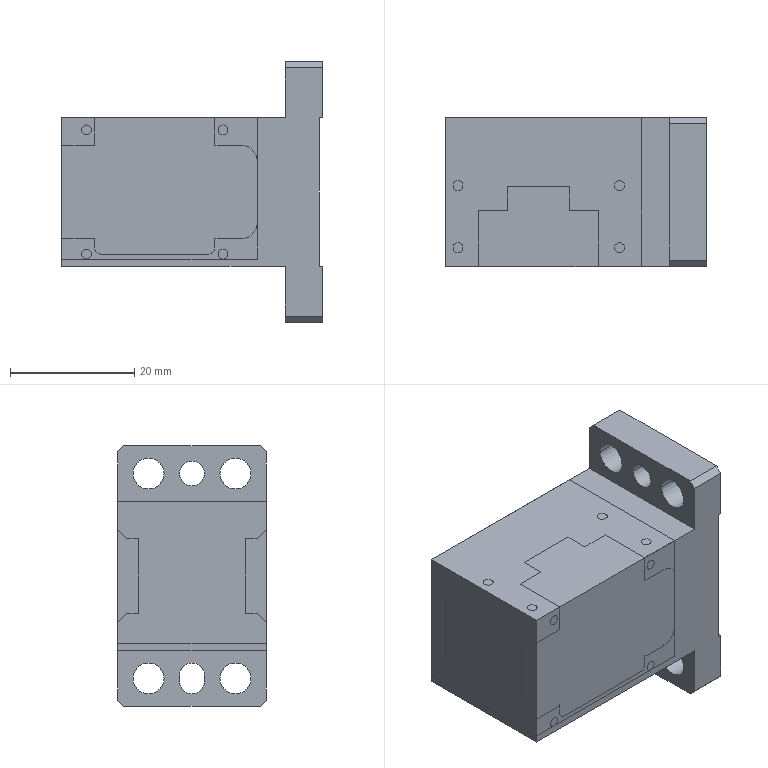NC program | NX | posted with a generic post | part box 42 x 24 x 42 mm
Lines 19 to 1216 of 4089:
(ZLEVEL_PROFILE , TOOL : D10)
N36 T10 M6
N38 G54
N40 G17 G0 G90 X26.1 Y11.429 B0. C0. S3000 M3
N42 G43 Z30. H10
N44 Z1.5
N46 G94 G1 Y-12. Z0.272 F1000.
N48 Y-12.554 Z0.243
N50 X25.766 Y-13.898 Z0.171
N52 X25.084 Y-15.104 Z0.098
N54 X24.104 Y-16.084 Z0.025
N56 X22.898 Y-16.766 Z-0.047
N58 X21.554 Y-17.1 Z-0.12
N60 X21. Z-0.149
N62 X-21. F1800.
N64 G2 X-26.1 Y-12. R5.1
N66 G1 Y12.
N68 G2 X-21. Y17.1 R5.1
N70 G1 X21.
N72 G2 X26.1 Y12. R5.1
N74 G1 Y-12.
N76 G2 X21. Y-17.1 R5.1
N78 G1 X12.467 Z-0.298
N80 X-21.
N82 G2 X-26.1 Y-12. R5.1
N84 G1 Y12.
N86 G2 X-21. Y17.1 R5.1
N88 G1 X21.
N90 G2 X26.1 Y12. R5.1
N92 G1 Y-12.
N94 G2 X21. Y-17.1 R5.1
N96 G1 X12.467 Z-0.447
N98 X-21.
N100 G2 X-26.1 Y-12. R5.1
N102 G1 Y12.
N104 G2 X-21. Y17.1 R5.1
N106 G1 X21.
N108 G2 X26.1 Y12. R5.1
N110 G1 Y-12.
N112 G2 X21. Y-17.1 R5.1
N114 G1 X12.467 Z-0.596
N116 X-21.
N118 G2 X-26.1 Y-12. R5.1
N120 G1 Y12.
N122 G2 X-21. Y17.1 R5.1
N124 G1 X21.
N126 G2 X26.1 Y12. R5.1
N128 G1 Y-12.
N130 G2 X21. Y-17.1 R5.1
N132 G1 X12.467 Z-0.745
N134 X-21.
N136 G2 X-26.1 Y-12. R5.1
N138 G1 Y12.
N140 G2 X-21. Y17.1 R5.1
N142 G1 X21.
N144 G2 X26.1 Y12. R5.1
N146 G1 Y-12.
N148 G2 X21. Y-17.1 R5.1
N150 G1 X12.467 Z-0.894
N152 X-21.
N154 G2 X-26.1 Y-12. R5.1
N156 G1 Y12.
N158 G2 X-21. Y17.1 R5.1
N160 G1 X21.
N162 G2 X26.1 Y12. R5.1
N164 G1 Y-12.
N166 G2 X21. Y-17.1 R5.1
N168 G1 X12.467 Z-1.043
N170 X-21.
N172 G2 X-26.1 Y-12. R5.1
N174 G1 Y12.
N176 G2 X-21. Y17.1 R5.1
N178 G1 X21.
N180 G2 X26.1 Y12. R5.1
N182 G1 Y-12.
N184 G2 X21. Y-17.1 R5.1
N186 G1 X12.467 Z-1.191
N188 X-21.
N190 G2 X-26.1 Y-12. R5.1
N192 G1 Y12.
N194 G2 X-21. Y17.1 R5.1
N196 G1 X21.
N198 G2 X26.1 Y12. R5.1
N200 G1 Y-12.
N202 G2 X21. Y-17.1 R5.1
N204 G1 X12.467 Z-1.34
N206 X-21.
N208 G2 X-26.1 Y-12. R5.1
N210 G1 Y12.
N212 G2 X-21. Y17.1 R5.1
N214 G1 X21.
N216 G2 X26.1 Y12. R5.1
N218 G1 Y-12.
N220 G2 X21. Y-17.1 R5.1
N222 G1 X12.467 Z-1.489
N224 X-21.
N226 G2 X-26.1 Y-12. R5.1
N228 G1 Y12.
N230 G2 X-21. Y17.1 R5.1
N232 G1 X21.
N234 G2 X26.1 Y12. R5.1
N236 G1 Y-12.
N238 G2 X21. Y-17.1 R5.1
N240 G1 X12.467 Z-1.638
N242 X-21.
N244 G2 X-26.1 Y-12. R5.1
N246 G1 Y12.
N248 G2 X-21. Y17.1 R5.1
N250 G1 X21.
N252 G2 X26.1 Y12. R5.1
N254 G1 Y-12.
N256 G2 X21. Y-17.1 R5.1
N258 G1 X12.467 Z-1.787
N260 X-21.
N262 G2 X-26.1 Y-12. R5.1
N264 G1 Y12.
N266 G2 X-21. Y17.1 R5.1
N268 G1 X21.
N270 G2 X26.1 Y12. R5.1
N272 G1 Y-12.
N274 G2 X21. Y-17.1 R5.1
N276 G1 X12.467 Z-1.936
N278 X-21.
N280 G2 X-26.1 Y-12. R5.1
N282 G1 Y12.
N284 G2 X-21. Y17.1 R5.1
N286 G1 X21.
N288 G2 X26.1 Y12. R5.1
N290 G1 Y-12.
N292 G2 X21. Y-17.1 R5.1
N294 G1 X12.467 Z-2.085
N296 X-21.
N298 G2 X-26.1 Y-12. R5.1
N300 G1 Y12.
N302 G2 X-21. Y17.1 R5.1
N304 G1 X21.
N306 G2 X26.1 Y12. R5.1
N308 G1 Y-12.
N310 G2 X21. Y-17.1 R5.1
N312 G1 X12.467 Z-2.234
N314 X-21.
N316 G2 X-26.1 Y-12. R5.1
N318 G1 Y12.
N320 G2 X-21. Y17.1 R5.1
N322 G1 X21.
N324 G2 X26.1 Y12. R5.1
N326 G1 Y-12.
N328 G2 X21. Y-17.1 R5.1
N330 G1 X12.467 Z-2.383
N332 X-21.
N334 G2 X-26.1 Y-12. R5.1
N336 G1 Y12.
N338 G2 X-21. Y17.1 R5.1
N340 G1 X21.
N342 G2 X26.1 Y12. R5.1
N344 G1 Y-12.
N346 G2 X21. Y-17.1 R5.1
N348 G1 X12.467 Z-2.532
N350 X-21.
N352 G2 X-26.1 Y-12. R5.1
N354 G1 Y12.
N356 G2 X-21. Y17.1 R5.1
N358 G1 X21.
N360 G2 X26.1 Y12. R5.1
N362 G1 Y-12.
N364 G2 X21. Y-17.1 R5.1
N366 G1 X12.467 Z-2.681
N368 X-21.
N370 G2 X-26.1 Y-12. R5.1
N372 G1 Y12.
N374 G2 X-21. Y17.1 R5.1
N376 G1 X21.
N378 G2 X26.1 Y12. R5.1
N380 G1 Y-12.
N382 G2 X21. Y-17.1 R5.1
N384 G1 X12.467 Z-2.83
N386 X-21.
N388 G2 X-26.1 Y-12. R5.1
N390 G1 Y12.
N392 G2 X-21. Y17.1 R5.1
N394 G1 X21.
N396 G2 X26.1 Y12. R5.1
N398 G1 Y-12.
N400 G2 X21. Y-17.1 R5.1
N402 G1 X12.467 Z-2.979
N404 X-21.
N406 G2 X-26.1 Y-12. R5.1
N408 G1 Y12.
N410 G2 X-21. Y17.1 R5.1
N412 G1 X21.
N414 G2 X26.1 Y12. R5.1
N416 G1 Y-12.
N418 G2 X21. Y-17.1 R5.1
N420 G1 X12.467 Z-3.128
N422 X-21.
N424 G2 X-26.1 Y-12. R5.1
N426 G1 Y12.
N428 G2 X-21. Y17.1 R5.1
N430 G1 X21.
N432 G2 X26.1 Y12. R5.1
N434 G1 Y-12.
N436 G2 X21. Y-17.1 R5.1
N438 G1 X12.467 Z-3.277
N440 X-21.
N442 G2 X-26.1 Y-12. R5.1
N444 G1 Y12.
N446 G2 X-21. Y17.1 R5.1
N448 G1 X21.
N450 G2 X26.1 Y12. R5.1
N452 G1 Y-12.
N454 G2 X21. Y-17.1 R5.1
N456 G1 X12.467 Z-3.426
N458 X-21.
N460 G2 X-26.1 Y-12. R5.1
N462 G1 Y12.
N464 G2 X-21. Y17.1 R5.1
N466 G1 X21.
N468 G2 X26.1 Y12. R5.1
N470 G1 Y-12.
N472 G2 X21. Y-17.1 R5.1
N474 G1 X12.467 Z-3.574
N476 X-21.
N478 G2 X-26.1 Y-12. R5.1
N480 G1 Y12.
N482 G2 X-21. Y17.1 R5.1
N484 G1 X21.
N486 G2 X26.1 Y12. R5.1
N488 G1 Y-12.
N490 G2 X21. Y-17.1 R5.1
N492 G1 X12.467 Z-3.723
N494 X-21.
N496 G2 X-26.1 Y-12. R5.1
N498 G1 Y12.
N500 G2 X-21. Y17.1 R5.1
N502 G1 X21.
N504 G2 X26.1 Y12. R5.1
N506 G1 Y-12.
N508 G2 X21. Y-17.1 R5.1
N510 G1 X12.467 Z-3.872
N512 X-21.
N514 G2 X-26.1 Y-12. R5.1
N516 G1 Y12.
N518 G2 X-21. Y17.1 R5.1
N520 G1 X21.
N522 G2 X26.1 Y12. R5.1
N524 G1 Y-12.
N526 G2 X21. Y-17.1 R5.1
N528 G1 X12.467 Z-4.021
N530 X-21.
N532 G2 X-26.1 Y-12. R5.1
N534 G1 Y12.
N536 G2 X-21. Y17.1 R5.1
N538 G1 X21.
N540 G2 X26.1 Y12. R5.1
N542 G1 Y-12.
N544 G2 X21. Y-17.1 R5.1
N546 G1 X12.467 Z-4.17
N548 X-21.
N550 G2 X-26.1 Y-12. R5.1
N552 G1 Y12.
N554 G2 X-21. Y17.1 R5.1
N556 G1 X21.
N558 G2 X26.1 Y12. R5.1
N560 G1 Y-12.
N562 G2 X21. Y-17.1 R5.1
N564 G1 X12.467 Z-4.319
N566 X-21.
N568 G2 X-26.1 Y-12. R5.1
N570 G1 Y12.
N572 G2 X-21. Y17.1 R5.1
N574 G1 X21.
N576 G2 X26.1 Y12. R5.1
N578 G1 Y-12.
N580 G2 X21. Y-17.1 R5.1
N582 G1 X12.467 Z-4.468
N584 X-21.
N586 G2 X-26.1 Y-12. R5.1
N588 G1 Y12.
N590 G2 X-21. Y17.1 R5.1
N592 G1 X21.
N594 G2 X26.1 Y12. R5.1
N596 G1 Y-12.
N598 G2 X21. Y-17.1 R5.1
N600 G1 X12.467 Z-4.617
N602 X-21.
N604 G2 X-26.1 Y-12. R5.1
N606 G1 Y12.
N608 G2 X-21. Y17.1 R5.1
N610 G1 X21.
N612 G2 X26.1 Y12. R5.1
N614 G1 Y-12.
N616 G2 X21. Y-17.1 R5.1
N618 G1 X12.467 Z-4.766
N620 X-21.
N622 G2 X-26.1 Y-12. R5.1
N624 G1 Y12.
N626 G2 X-21. Y17.1 R5.1
N628 G1 X21.
N630 G2 X26.1 Y12. R5.1
N632 G1 Y-12.
N634 G2 X21. Y-17.1 R5.1
N636 G1 X12.467 Z-4.915
N638 X-21.
N640 G2 X-26.1 Y-12. R5.1
N642 G1 Y12.
N644 G2 X-21. Y17.1 R5.1
N646 G1 X21.
N648 G2 X26.1 Y12. R5.1
N650 G1 Y-12.
N652 G2 X21. Y-17.1 R5.1
N654 G1 X12.467 Z-5.064
N656 X-21.
N658 G2 X-26.1 Y-12. R5.1
N660 G1 Y12.
N662 G2 X-21. Y17.1 R5.1
N664 G1 X21.
N666 G2 X26.1 Y12. R5.1
N668 G1 Y-12.
N670 G2 X21. Y-17.1 R5.1
N672 G1 X12.467 Z-5.213
N674 X-21.
N676 G2 X-26.1 Y-12. R5.1
N678 G1 Y12.
N680 G2 X-21. Y17.1 R5.1
N682 G1 X21.
N684 G2 X26.1 Y12. R5.1
N686 G1 Y-12.
N688 G2 X21. Y-17.1 R5.1
N690 G1 X12.467 Z-5.362
N692 X-21.
N694 G2 X-26.1 Y-12. R5.1
N696 G1 Y12.
N698 G2 X-21. Y17.1 R5.1
N700 G1 X21.
N702 G2 X26.1 Y12. R5.1
N704 G1 Y-12.
N706 G2 X21. Y-17.1 R5.1
N708 G1 X12.467 Z-5.511
N710 X-21.
N712 G2 X-26.1 Y-12. R5.1
N714 G1 Y12.
N716 G2 X-21. Y17.1 R5.1
N718 G1 X21.
N720 G2 X26.1 Y12. R5.1
N722 G1 Y-12.
N724 G2 X21. Y-17.1 R5.1
N726 G1 X12.467 Z-5.66
N728 X-21.
N730 G2 X-26.1 Y-12. R5.1
N732 G1 Y12.
N734 G2 X-21. Y17.1 R5.1
N736 G1 X21.
N738 G2 X26.1 Y12. R5.1
N740 G1 Y-12.
N742 G2 X21. Y-17.1 R5.1
N744 G1 X12.467 Z-5.809
N746 X-21.
N748 G2 X-26.1 Y-12. R5.1
N750 G1 Y12.
N752 G2 X-21. Y17.1 R5.1
N754 G1 X21.
N756 G2 X26.1 Y12. R5.1
N758 G1 Y-12.
N760 G2 X21. Y-17.1 R5.1
N762 G1 X12.467 Z-5.957
N764 X-21.
N766 G2 X-26.1 Y-12. R5.1
N768 G1 Y12.
N770 G2 X-21. Y17.1 R5.1
N772 G1 X21.
N774 G2 X26.1 Y12. R5.1
N776 G1 Y-12.
N778 G2 X21. Y-17.1 R5.1
N780 G1 X12.467 Z-6.106
N782 X-21.
N784 G2 X-26.1 Y-12. R5.1
N786 G1 Y12.
N788 G2 X-21. Y17.1 R5.1
N790 G1 X21.
N792 G2 X26.1 Y12. R5.1
N794 G1 Y-12.
N796 G2 X21. Y-17.1 R5.1
N798 G1 X12.467 Z-6.255
N800 X-21.
N802 G2 X-26.1 Y-12. R5.1
N804 G1 Y12.
N806 G2 X-21. Y17.1 R5.1
N808 G1 X21.
N810 G2 X26.1 Y12. R5.1
N812 G1 Y-12.
N814 G2 X21. Y-17.1 R5.1
N816 G1 X12.467 Z-6.404
N818 X-21.
N820 G2 X-26.1 Y-12. R5.1
N822 G1 Y12.
N824 G2 X-21. Y17.1 R5.1
N826 G1 X21.
N828 G2 X26.1 Y12. R5.1
N830 G1 Y-12.
N832 G2 X21. Y-17.1 R5.1
N834 G1 X12.467 Z-6.553
N836 X-21.
N838 G2 X-26.1 Y-12. R5.1
N840 G1 Y12.
N842 G2 X-21. Y17.1 R5.1
N844 G1 X21.
N846 G2 X26.1 Y12. R5.1
N848 G1 Y-12.
N850 G2 X21. Y-17.1 R5.1
N852 G1 X12.467 Z-6.702
N854 X-21.
N856 G2 X-26.1 Y-12. R5.1
N858 G1 Y12.
N860 G2 X-21. Y17.1 R5.1
N862 G1 X21.
N864 G2 X26.1 Y12. R5.1
N866 G1 Y-12.
N868 G2 X21. Y-17.1 R5.1
N870 G1 X12.467 Z-6.851
N872 X-21.
N874 G2 X-26.1 Y-12. R5.1
N876 G1 Y12.
N878 G2 X-21. Y17.1 R5.1
N880 G1 X21.
N882 G2 X26.1 Y12. R5.1
N884 G1 Y-12.
N886 G2 X21. Y-17.1 R5.1
N888 G1 X12.467 Z-7.
N890 X-21.
N892 G2 X-26.1 Y-12. R5.1
N894 G1 Y12.
N896 G2 X-21. Y17.1 R5.1
N898 G1 X21.
N900 G2 X26.1 Y12. R5.1
N902 G1 Y-12.
N904 G2 X21. Y-17.1 R5.1
N906 G1 X12.406 Z-7.15
N908 X-21.
N910 G2 X-26.1 Y-12. R5.1
N912 G1 Y12.
N914 G2 X-21. Y17.1 R5.1
N916 G1 X21.
N918 G2 X26.1 Y12. R5.1
N920 G1 Y-12.
N922 G2 X21. Y-17.1 R5.1
N924 G1 X12.406 Z-7.3
N926 X-21.
N928 G2 X-26.1 Y-12. R5.1
N930 G1 Y12.
N932 G2 X-21. Y17.1 R5.1
N934 G1 X21.
N936 G2 X26.1 Y12. R5.1
N938 G1 Y-12.
N940 G2 X21. Y-17.1 R5.1
N942 G1 X12.406 Z-7.45
N944 X-21.
N946 G2 X-26.1 Y-12. R5.1
N948 G1 Y12.
N950 G2 X-21. Y17.1 R5.1
N952 G1 X21.
N954 G2 X26.1 Y12. R5.1
N956 G1 Y-12.
N958 G2 X21. Y-17.1 R5.1
N960 G1 X12.406 Z-7.6
N962 X-21.
N964 G2 X-26.1 Y-12. R5.1
N966 G1 Y12.
N968 G2 X-21. Y17.1 R5.1
N970 G1 X21.
N972 G2 X26.1 Y12. R5.1
N974 G1 Y-12.
N976 G2 X21. Y-17.1 R5.1
N978 G1 X12.406 Z-7.75
N980 X-21.
N982 G2 X-26.1 Y-12. R5.1
N984 G1 Y12.
N986 G2 X-21. Y17.1 R5.1
N988 G1 X21.
N990 G2 X26.1 Y12. R5.1
N992 G1 Y-12.
N994 G2 X21. Y-17.1 R5.1
N996 G1 X12.406 Z-7.9
N998 X-21.
N1000 G2 X-26.1 Y-12. R5.1
N1002 G1 Y12.
N1004 G2 X-21. Y17.1 R5.1
N1006 G1 X21.
N1008 G2 X26.1 Y12. R5.1
N1010 G1 Y-12.
N1012 G2 X21. Y-17.1 R5.1
N1014 G1 X12.406 Z-8.05
N1016 X-21.
N1018 G2 X-26.1 Y-12. R5.1
N1020 G1 Y12.
N1022 G2 X-21. Y17.1 R5.1
N1024 G1 X21.
N1026 G2 X26.1 Y12. R5.1
N1028 G1 Y-12.
N1030 G2 X21. Y-17.1 R5.1
N1032 G1 X12.406 Z-8.2
N1034 X-21.
N1036 G2 X-26.1 Y-12. R5.1
N1038 G1 Y12.
N1040 G2 X-21. Y17.1 R5.1
N1042 G1 X21.
N1044 G2 X26.1 Y12. R5.1
N1046 G1 Y-12.
N1048 G2 X21. Y-17.1 R5.1
N1050 G1 X12.406 Z-8.35
N1052 X-21.
N1054 G2 X-26.1 Y-12. R5.1
N1056 G1 Y12.
N1058 G2 X-21. Y17.1 R5.1
N1060 G1 X21.
N1062 G2 X26.1 Y12. R5.1
N1064 G1 Y-12.
N1066 G2 X21. Y-17.1 R5.1
N1068 G1 X12.406 Z-8.5
N1070 X-21.
N1072 G2 X-26.1 Y-12. R5.1
N1074 G1 Y12.
N1076 G2 X-21. Y17.1 R5.1
N1078 G1 X21.
N1080 G2 X26.1 Y12. R5.1
N1082 G1 Y-12.
N1084 G2 X21. Y-17.1 R5.1
N1086 G1 X12.406 Z-8.65
N1088 X-21.
N1090 G2 X-26.1 Y-12. R5.1
N1092 G1 Y12.
N1094 G2 X-21. Y17.1 R5.1
N1096 G1 X21.
N1098 G2 X26.1 Y12. R5.1
N1100 G1 Y-12.
N1102 G2 X21. Y-17.1 R5.1
N1104 G1 X12.406 Z-8.8
N1106 X-21.
N1108 G2 X-26.1 Y-12. R5.1
N1110 G1 Y12.
N1112 G2 X-21. Y17.1 R5.1
N1114 G1 X21.
N1116 G2 X26.1 Y12. R5.1
N1118 G1 Y-12.
N1120 G2 X21. Y-17.1 R5.1
N1122 G1 X12.406 Z-8.95
N1124 X-21.
N1126 G2 X-26.1 Y-12. R5.1
N1128 G1 Y12.
N1130 G2 X-21. Y17.1 R5.1
N1132 G1 X21.
N1134 G2 X26.1 Y12. R5.1
N1136 G1 Y-12.
N1138 G2 X21. Y-17.1 R5.1
N1140 G1 X12.406 Z-9.1
N1142 X-21.
N1144 G2 X-26.1 Y-12. R5.1
N1146 G1 Y12.
N1148 G2 X-21. Y17.1 R5.1
N1150 G1 X21.
N1152 G2 X26.1 Y12. R5.1
N1154 G1 Y-12.
N1156 G2 X21. Y-17.1 R5.1
N1158 G1 X12.406 Z-9.25
N1160 X-21.
N1162 G2 X-26.1 Y-12. R5.1
N1164 G1 Y12.
N1166 G2 X-21. Y17.1 R5.1
N1168 G1 X21.
N1170 G2 X26.1 Y12. R5.1
N1172 G1 Y-12.
N1174 G2 X21. Y-17.1 R5.1
N1176 G1 X12.406 Z-9.4
N1178 X-21.
N1180 G2 X-26.1 Y-12. R5.1
N1182 G1 Y12.
N1184 G2 X-21. Y17.1 R5.1
N1186 G1 X21.
N1188 G2 X26.1 Y12. R5.1
N1190 G1 Y-12.
N1192 G2 X21. Y-17.1 R5.1
N1194 G1 X12.406 Z-9.55
N1196 X-21.
N1198 G2 X-26.1 Y-12. R5.1
N1200 G1 Y12.
N1202 G2 X-21. Y17.1 R5.1
N1204 G1 X21.
N1206 G2 X26.1 Y12. R5.1
N1208 G1 Y-12.
N1210 G2 X21. Y-17.1 R5.1
N1212 G1 X12.406 Z-9.7
N1214 X-21.
N1216 G2 X-26.1 Y-12. R5.1
N1218 G1 Y12.
N1220 G2 X-21. Y17.1 R5.1
N1222 G1 X21.
N1224 G2 X26.1 Y12. R5.1
N1226 G1 Y-12.
N1228 G2 X21. Y-17.1 R5.1
N1230 G1 X12.406 Z-9.85
N1232 X-21.
N1234 G2 X-26.1 Y-12. R5.1
N1236 G1 Y12.
N1238 G2 X-21. Y17.1 R5.1
N1240 G1 X21.
N1242 G2 X26.1 Y12. R5.1
N1244 G1 Y-12.
N1246 G2 X21. Y-17.1 R5.1
N1248 G1 X12.406 Z-10.
N1250 X-21.
N1252 G2 X-26.1 Y-12. R5.1
N1254 G1 Y12.
N1256 G2 X-21. Y17.1 R5.1
N1258 G1 X21.
N1260 G2 X26.1 Y12. R5.1
N1262 G1 Y-12.
N1264 G2 X21. Y-17.1 R5.1
N1266 G1 X12.406 Z-10.15
N1268 X-21.
N1270 G2 X-26.1 Y-12. R5.1
N1272 G1 Y12.
N1274 G2 X-21. Y17.1 R5.1
N1276 G1 X21.
N1278 G2 X26.1 Y12. R5.1
N1280 G1 Y-12.
N1282 G2 X21. Y-17.1 R5.1
N1284 G1 X12.406 Z-10.3
N1286 X-21.
N1288 G2 X-26.1 Y-12. R5.1
N1290 G1 Y12.
N1292 G2 X-21. Y17.1 R5.1
N1294 G1 X21.
N1296 G2 X26.1 Y12. R5.1
N1298 G1 Y-12.
N1300 G2 X21. Y-17.1 R5.1
N1302 G1 X12.406 Z-10.45
N1304 X-21.
N1306 G2 X-26.1 Y-12. R5.1
N1308 G1 Y12.
N1310 G2 X-21. Y17.1 R5.1
N1312 G1 X21.
N1314 G2 X26.1 Y12. R5.1
N1316 G1 Y-12.
N1318 G2 X21. Y-17.1 R5.1
N1320 G1 X12.406 Z-10.6
N1322 X-21.
N1324 G2 X-26.1 Y-12. R5.1
N1326 G1 Y12.
N1328 G2 X-21. Y17.1 R5.1
N1330 G1 X21.
N1332 G2 X26.1 Y12. R5.1
N1334 G1 Y-12.
N1336 G2 X21. Y-17.1 R5.1
N1338 G1 X12.406 Z-10.75
N1340 X-21.
N1342 G2 X-26.1 Y-12. R5.1
N1344 G1 Y12.
N1346 G2 X-21. Y17.1 R5.1
N1348 G1 X21.
N1350 G2 X26.1 Y12. R5.1
N1352 G1 Y-12.
N1354 G2 X21. Y-17.1 R5.1
N1356 G1 X12.406 Z-10.9
N1358 X-21.
N1360 G2 X-26.1 Y-12. R5.1
N1362 G1 Y12.
N1364 G2 X-21. Y17.1 R5.1
N1366 G1 X21.
N1368 G2 X26.1 Y12. R5.1
N1370 G1 Y-12.
N1372 G2 X21. Y-17.1 R5.1
N1374 G1 X12.406 Z-11.05
N1376 X-21.
N1378 G2 X-26.1 Y-12. R5.1
N1380 G1 Y12.
N1382 G2 X-21. Y17.1 R5.1
N1384 G1 X21.
N1386 G2 X26.1 Y12. R5.1
N1388 G1 Y-12.
N1390 G2 X21. Y-17.1 R5.1
N1392 G1 X12.406 Z-11.2
N1394 X-21.
N1396 G2 X-26.1 Y-12. R5.1
N1398 G1 Y12.
N1400 G2 X-21. Y17.1 R5.1
N1402 G1 X21.
N1404 G2 X26.1 Y12. R5.1
N1406 G1 Y-12.
N1408 G2 X21. Y-17.1 R5.1
N1410 G1 X12.406 Z-11.35
N1412 X-21.
N1414 G2 X-26.1 Y-12. R5.1
N1416 G1 Y12.
N1418 G2 X-21. Y17.1 R5.1
N1420 G1 X21.
N1422 G2 X26.1 Y12. R5.1
N1424 G1 Y-12.
N1426 G2 X21. Y-17.1 R5.1
N1428 G1 X12.406 Z-11.5
N1430 X-21.
N1432 G2 X-26.1 Y-12. R5.1
N1434 G1 Y12.
N1436 G2 X-21. Y17.1 R5.1
N1438 G1 X21.
N1440 G2 X26.1 Y12. R5.1
N1442 G1 Y-12.
N1444 G2 X21. Y-17.1 R5.1
N1446 G1 X12.406 Z-11.65
N1448 X-21.
N1450 G2 X-26.1 Y-12. R5.1
N1452 G1 Y12.
N1454 G2 X-21. Y17.1 R5.1
N1456 G1 X21.
N1458 G2 X26.1 Y12. R5.1
N1460 G1 Y-12.
N1462 G2 X21. Y-17.1 R5.1
N1464 G1 X12.406 Z-11.8
N1466 X-21.
N1468 G2 X-26.1 Y-12. R5.1
N1470 G1 Y12.
N1472 G2 X-21. Y17.1 R5.1
N1474 G1 X21.
N1476 G2 X26.1 Y12. R5.1
N1478 G1 Y-12.
N1480 G2 X21. Y-17.1 R5.1
N1482 G1 X12.406 Z-11.95
N1484 X-21.
N1486 G2 X-26.1 Y-12. R5.1
N1488 G1 Y12.
N1490 G2 X-21. Y17.1 R5.1
N1492 G1 X21.
N1494 G2 X26.1 Y12. R5.1
N1496 G1 Y-12.
N1498 G2 X21. Y-17.1 R5.1
N1500 G1 X12.406 Z-12.1
N1502 X-21.
N1504 G2 X-26.1 Y-12. R5.1
N1506 G1 Y12.
N1508 G2 X-21. Y17.1 R5.1
N1510 G1 X21.
N1512 G2 X26.1 Y12. R5.1
N1514 G1 Y-12.
N1516 G2 X21. Y-17.1 R5.1
N1518 G1 X12.406 Z-12.25
N1520 X-21.
N1522 G2 X-26.1 Y-12. R5.1
N1524 G1 Y12.
N1526 G2 X-21. Y17.1 R5.1
N1528 G1 X21.
N1530 G2 X26.1 Y12. R5.1
N1532 G1 Y-12.
N1534 G2 X21. Y-17.1 R5.1
N1536 G1 X12.406 Z-12.4
N1538 X-21.
N1540 G2 X-26.1 Y-12. R5.1
N1542 G1 Y12.
N1544 G2 X-21. Y17.1 R5.1
N1546 G1 X21.
N1548 G2 X26.1 Y12. R5.1
N1550 G1 Y-12.
N1552 G2 X21. Y-17.1 R5.1
N1554 G1 X12.406 Z-12.55
N1556 X-21.
N1558 G2 X-26.1 Y-12. R5.1
N1560 G1 Y12.
N1562 G2 X-21. Y17.1 R5.1
N1564 G1 X21.
N1566 G2 X26.1 Y12. R5.1
N1568 G1 Y-12.
N1570 G2 X21. Y-17.1 R5.1
N1572 G1 X12.406 Z-12.7
N1574 X-21.
N1576 G2 X-26.1 Y-12. R5.1
N1578 G1 Y12.
N1580 G2 X-21. Y17.1 R5.1
N1582 G1 X21.
N1584 G2 X26.1 Y12. R5.1
N1586 G1 Y-12.
N1588 G2 X21. Y-17.1 R5.1
N1590 G1 X12.406 Z-12.85
N1592 X-21.
N1594 G2 X-26.1 Y-12. R5.1
N1596 G1 Y12.
N1598 G2 X-21. Y17.1 R5.1
N1600 G1 X21.
N1602 G2 X26.1 Y12. R5.1
N1604 G1 Y-12.
N1606 G2 X21. Y-17.1 R5.1
N1608 G1 X12.406 Z-13.
N1610 X-21.
N1612 G2 X-26.1 Y-12. R5.1
N1614 G1 Y12.
N1616 G2 X-21. Y17.1 R5.1
N1618 G1 X21.
N1620 G2 X26.1 Y12. R5.1
N1622 G1 Y-12.
N1624 G2 X21. Y-17.1 R5.1
N1626 G1 X12.436 Z-13.149
N1628 X-21.
N1630 G2 X-26.1 Y-12. R5.1
N1632 G1 Y12.
N1634 G2 X-21. Y17.1 R5.1
N1636 G1 X21.
N1638 G2 X26.1 Y12. R5.1
N1640 G1 Y-12.
N1642 G2 X21. Y-17.1 R5.1
N1644 G1 X12.436 Z-13.299
N1646 X-21.
N1648 G2 X-26.1 Y-12. R5.1
N1650 G1 Y12.
N1652 G2 X-21. Y17.1 R5.1
N1654 G1 X21.
N1656 G2 X26.1 Y12. R5.1
N1658 G1 Y-12.
N1660 G2 X21. Y-17.1 R5.1
N1662 G1 X12.436 Z-13.448
N1664 X-21.
N1666 G2 X-26.1 Y-12. R5.1
N1668 G1 Y12.
N1670 G2 X-21. Y17.1 R5.1
N1672 G1 X21.
N1674 G2 X26.1 Y12. R5.1
N1676 G1 Y-12.
N1678 G2 X21. Y-17.1 R5.1
N1680 G1 X12.436 Z-13.598
N1682 X-21.
N1684 G2 X-26.1 Y-12. R5.1
N1686 G1 Y12.
N1688 G2 X-21. Y17.1 R5.1
N1690 G1 X21.
N1692 G2 X26.1 Y12. R5.1
N1694 G1 Y-12.
N1696 G2 X21. Y-17.1 R5.1
N1698 G1 X12.436 Z-13.747
N1700 X-21.
N1702 G2 X-26.1 Y-12. R5.1
N1704 G1 Y12.
N1706 G2 X-21. Y17.1 R5.1
N1708 G1 X21.
N1710 G2 X26.1 Y12. R5.1
N1712 G1 Y-12.
N1714 G2 X21. Y-17.1 R5.1
N1716 G1 X12.436 Z-13.897
N1718 X-21.
N1720 G2 X-26.1 Y-12. R5.1
N1722 G1 Y12.
N1724 G2 X-21. Y17.1 R5.1
N1726 G1 X21.
N1728 G2 X26.1 Y12. R5.1
N1730 G1 Y-12.
N1732 G2 X21. Y-17.1 R5.1
N1734 G1 X12.436 Z-14.046
N1736 X-21.
N1738 G2 X-26.1 Y-12. R5.1
N1740 G1 Y12.
N1742 G2 X-21. Y17.1 R5.1
N1744 G1 X21.
N1746 G2 X26.1 Y12. R5.1
N1748 G1 Y-12.
N1750 G2 X21. Y-17.1 R5.1
N1752 G1 X12.436 Z-14.196
N1754 X-21.
N1756 G2 X-26.1 Y-12. R5.1
N1758 G1 Y12.
N1760 G2 X-21. Y17.1 R5.1
N1762 G1 X21.
N1764 G2 X26.1 Y12. R5.1
N1766 G1 Y-12.
N1768 G2 X21. Y-17.1 R5.1
N1770 G1 X12.436 Z-14.345
N1772 X-21.
N1774 G2 X-26.1 Y-12. R5.1
N1776 G1 Y12.
N1778 G2 X-21. Y17.1 R5.1
N1780 G1 X21.
N1782 G2 X26.1 Y12. R5.1
N1784 G1 Y-12.
N1786 G2 X21. Y-17.1 R5.1
N1788 G1 X12.436 Z-14.495
N1790 X-21.
N1792 G2 X-26.1 Y-12. R5.1
N1794 G1 Y12.
N1796 G2 X-21. Y17.1 R5.1
N1798 G1 X21.
N1800 G2 X26.1 Y12. R5.1
N1802 G1 Y-12.
N1804 G2 X21. Y-17.1 R5.1
N1806 G1 X12.436 Z-14.644
N1808 X-21.
N1810 G2 X-26.1 Y-12. R5.1
N1812 G1 Y12.
N1814 G2 X-21. Y17.1 R5.1
N1816 G1 X21.
N1818 G2 X26.1 Y12. R5.1
N1820 G1 Y-12.
N1822 G2 X21. Y-17.1 R5.1
N1824 G1 X12.436 Z-14.794
N1826 X-21.
N1828 G2 X-26.1 Y-12. R5.1
N1830 G1 Y12.
N1832 G2 X-21. Y17.1 R5.1
N1834 G1 X21.
N1836 G2 X26.1 Y12. R5.1
N1838 G1 Y-12.
N1840 G2 X21. Y-17.1 R5.1
N1842 G1 X12.436 Z-14.943
N1844 X-21.
N1846 G2 X-26.1 Y-12. R5.1
N1848 G1 Y12.
N1850 G2 X-21. Y17.1 R5.1
N1852 G1 X21.
N1854 G2 X26.1 Y12. R5.1
N1856 G1 Y-12.
N1858 G2 X21. Y-17.1 R5.1
N1860 G1 X12.436 Z-15.093
N1862 X-21.
N1864 G2 X-26.1 Y-12. R5.1
N1866 G1 Y12.
N1868 G2 X-21. Y17.1 R5.1
N1870 G1 X21.
N1872 G2 X26.1 Y12. R5.1
N1874 G1 Y-12.
N1876 G2 X21. Y-17.1 R5.1
N1878 G1 X12.436 Z-15.242
N1880 X-21.
N1882 G2 X-26.1 Y-12. R5.1
N1884 G1 Y12.
N1886 G2 X-21. Y17.1 R5.1
N1888 G1 X21.
N1890 G2 X26.1 Y12. R5.1
N1892 G1 Y-12.
N1894 G2 X21. Y-17.1 R5.1
N1896 G1 X12.436 Z-15.392
N1898 X-21.
N1900 G2 X-26.1 Y-12. R5.1
N1902 G1 Y12.
N1904 G2 X-21. Y17.1 R5.1
N1906 G1 X21.
N1908 G2 X26.1 Y12. R5.1
N1910 G1 Y-12.
N1912 G2 X21. Y-17.1 R5.1
N1914 G1 X12.436 Z-15.541
N1916 X-21.
N1918 G2 X-26.1 Y-12. R5.1
N1920 G1 Y12.
N1922 G2 X-21. Y17.1 R5.1
N1924 G1 X21.
N1926 G2 X26.1 Y12. R5.1
N1928 G1 Y-12.
N1930 G2 X21. Y-17.1 R5.1
N1932 G1 X12.436 Z-15.691
N1934 X-21.
N1936 G2 X-26.1 Y-12. R5.1
N1938 G1 Y12.
N1940 G2 X-21. Y17.1 R5.1
N1942 G1 X21.
N1944 G2 X26.1 Y12. R5.1
N1946 G1 Y-12.
N1948 G2 X21. Y-17.1 R5.1
N1950 G1 X12.436 Z-15.84
N1952 X-21.
N1954 G2 X-26.1 Y-12. R5.1
N1956 G1 Y12.
N1958 G2 X-21. Y17.1 R5.1
N1960 G1 X21.
N1962 G2 X26.1 Y12. R5.1
N1964 G1 Y-12.
N1966 G2 X21. Y-17.1 R5.1
N1968 G1 X12.436 Z-15.99
N1970 X-21.
N1972 G2 X-26.1 Y-12. R5.1
N1974 G1 Y12.
N1976 G2 X-21. Y17.1 R5.1
N1978 G1 X21.
N1980 G2 X26.1 Y12. R5.1
N1982 G1 Y-12.
N1984 G2 X21. Y-17.1 R5.1
N1986 G1 X12.436 Z-16.139
N1988 X-21.
N1990 G2 X-26.1 Y-12. R5.1
N1992 G1 Y12.
N1994 G2 X-21. Y17.1 R5.1
N1996 G1 X21.
N1998 G2 X26.1 Y12. R5.1
N2000 G1 Y-12.
N2002 G2 X21. Y-17.1 R5.1
N2004 G1 X12.436 Z-16.289
N2006 X-21.
N2008 G2 X-26.1 Y-12. R5.1
N2010 G1 Y12.
N2012 G2 X-21. Y17.1 R5.1
N2014 G1 X21.
N2016 G2 X26.1 Y12. R5.1
N2018 G1 Y-12.
N2020 G2 X21. Y-17.1 R5.1
N2022 G1 X12.436 Z-16.438
N2024 X-21.
N2026 G2 X-26.1 Y-12. R5.1
N2028 G1 Y12.
N2030 G2 X-21. Y17.1 R5.1
N2032 G1 X21.
N2034 G2 X26.1 Y12. R5.1
N2036 G1 Y-12.
N2038 G2 X21. Y-17.1 R5.1
N2040 G1 X12.436 Z-16.588
N2042 X-21.
N2044 G2 X-26.1 Y-12. R5.1
N2046 G1 Y12.
N2048 G2 X-21. Y17.1 R5.1
N2050 G1 X21.
N2052 G2 X26.1 Y12. R5.1
N2054 G1 Y-12.
N2056 G2 X21. Y-17.1 R5.1
N2058 G1 X12.436 Z-16.737
N2060 X-21.
N2062 G2 X-26.1 Y-12. R5.1
N2064 G1 Y12.
N2066 G2 X-21. Y17.1 R5.1
N2068 G1 X21.
N2070 G2 X26.1 Y12. R5.1
N2072 G1 Y-12.
N2074 G2 X21. Y-17.1 R5.1
N2076 G1 X12.436 Z-16.887
N2078 X-21.
N2080 G2 X-26.1 Y-12. R5.1
N2082 G1 Y12.
N2084 G2 X-21. Y17.1 R5.1
N2086 G1 X21.
N2088 G2 X26.1 Y12. R5.1
N2090 G1 Y-12.
N2092 G2 X21. Y-17.1 R5.1
N2094 G1 X12.436 Z-17.036
N2096 X-21.
N2098 G2 X-26.1 Y-12. R5.1
N2100 G1 Y12.
N2102 G2 X-21. Y17.1 R5.1
N2104 G1 X21.
N2106 G2 X26.1 Y12. R5.1
N2108 G1 Y-12.
N2110 G2 X21. Y-17.1 R5.1
N2112 G1 X12.436 Z-17.186
N2114 X-21.
N2116 G2 X-26.1 Y-12. R5.1
N2118 G1 Y12.
N2120 G2 X-21. Y17.1 R5.1
N2122 G1 X21.
N2124 G2 X26.1 Y12. R5.1
N2126 G1 Y-12.
N2128 G2 X21. Y-17.1 R5.1
N2130 G1 X12.436 Z-17.335
N2132 X-21.
N2134 G2 X-26.1 Y-12. R5.1
N2136 G1 Y12.
N2138 G2 X-21. Y17.1 R5.1
N2140 G1 X21.
N2142 G2 X26.1 Y12. R5.1
N2144 G1 Y-12.
N2146 G2 X21. Y-17.1 R5.1
N2148 G1 X12.436 Z-17.485
N2150 X-21.
N2152 G2 X-26.1 Y-12. R5.1
N2154 G1 Y12.
N2156 G2 X-21. Y17.1 R5.1
N2158 G1 X21.
N2160 G2 X26.1 Y12. R5.1
N2162 G1 Y-12.
N2164 G2 X21. Y-17.1 R5.1
N2166 G1 X12.436 Z-17.634
N2168 X-21.
N2170 G2 X-26.1 Y-12. R5.1
N2172 G1 Y12.
N2174 G2 X-21. Y17.1 R5.1
N2176 G1 X21.
N2178 G2 X26.1 Y12. R5.1
N2180 G1 Y-12.
N2182 G2 X21. Y-17.1 R5.1
N2184 G1 X12.436 Z-17.784
N2186 X-21.
N2188 G2 X-26.1 Y-12. R5.1
N2190 G1 Y12.
N2192 G2 X-21. Y17.1 R5.1
N2194 G1 X21.
N2196 G2 X26.1 Y12. R5.1
N2198 G1 Y-12.
N2200 G2 X21. Y-17.1 R5.1
N2202 G1 X12.436 Z-17.933
N2204 X-21.
N2206 G2 X-26.1 Y-12. R5.1
N2208 G1 Y12.
N2210 G2 X-21. Y17.1 R5.1
N2212 G1 X21.
N2214 G2 X26.1 Y12. R5.1
N2216 G1 Y-12.
N2218 G2 X21. Y-17.1 R5.1
N2220 G1 X12.436 Z-18.082
N2222 X-21.
N2224 G2 X-26.1 Y-12. R5.1
N2226 G1 Y12.
N2228 G2 X-21. Y17.1 R5.1
N2230 G1 X21.
N2232 G2 X26.1 Y12. R5.1
N2234 G1 Y-12.
N2236 G2 X21. Y-17.1 R5.1
N2238 G1 X12.436 Z-18.232
N2240 X-21.
N2242 G2 X-26.1 Y-12. R5.1
N2244 G1 Y12.
N2246 G2 X-21. Y17.1 R5.1
N2248 G1 X21.
N2250 G2 X26.1 Y12. R5.1
N2252 G1 Y-12.
N2254 G2 X21. Y-17.1 R5.1
N2256 G1 X12.436 Z-18.381
N2258 X-21.
N2260 G2 X-26.1 Y-12. R5.1
N2262 G1 Y12.
N2264 G2 X-21. Y17.1 R5.1
N2266 G1 X21.
N2268 G2 X26.1 Y12. R5.1
N2270 G1 Y-12.
N2272 G2 X21. Y-17.1 R5.1
N2274 G1 X12.436 Z-18.531
N2276 X-21.
N2278 G2 X-26.1 Y-12. R5.1
N2280 G1 Y12.
N2282 G2 X-21. Y17.1 R5.1
N2284 G1 X21.
N2286 G2 X26.1 Y12. R5.1
N2288 G1 Y-12.
N2290 G2 X21. Y-17.1 R5.1
N2292 G1 X12.436 Z-18.68
N2294 X-21.
N2296 G2 X-26.1 Y-12. R5.1
N2298 G1 Y12.
N2300 G2 X-21. Y17.1 R5.1
N2302 G1 X21.
N2304 G2 X26.1 Y12. R5.1
N2306 G1 Y-12.
N2308 G2 X21. Y-17.1 R5.1
N2310 G1 X12.436 Z-18.83
N2312 X-21.
N2314 G2 X-26.1 Y-12. R5.1
N2316 G1 Y12.
N2318 G2 X-21. Y17.1 R5.1
N2320 G1 X21.
N2322 G2 X26.1 Y12. R5.1
N2324 G1 Y-12.
N2326 G2 X21. Y-17.1 R5.1
N2328 G1 X12.436 Z-18.979
N2330 X-21.
N2332 G2 X-26.1 Y-12. R5.1
N2334 G1 Y12.
N2336 G2 X-21. Y17.1 R5.1
N2338 G1 X21.
N2340 G2 X26.1 Y12. R5.1
N2342 G1 Y-12.
N2344 G2 X21. Y-17.1 R5.1
N2346 G1 X12.436 Z-19.129
N2348 X-21.
N2350 G2 X-26.1 Y-12. R5.1
N2352 G1 Y12.
N2354 G2 X-21. Y17.1 R5.1
N2356 G1 X21.
N2358 G2 X26.1 Y12. R5.1
N2360 G1 Y-12.
N2362 G2 X21. Y-17.1 R5.1
N2364 G1 X12.436 Z-19.278
N2366 X-21.
N2368 G2 X-26.1 Y-12. R5.1
N2370 G1 Y12.
N2372 G2 X-21. Y17.1 R5.1
N2374 G1 X21.
N2376 G2 X26.1 Y12. R5.1
N2378 G1 Y-12.
N2380 G2 X21. Y-17.1 R5.1
N2382 G1 X12.436 Z-19.428
N2384 X-21.
N2386 G2 X-26.1 Y-12. R5.1
N2388 G1 Y12.
N2390 G2 X-21. Y17.1 R5.1
N2392 G1 X21.
N2394 G2 X26.1 Y12. R5.1
N2396 G1 Y-12.
N2398 G2 X21. Y-17.1 R5.1
N2400 G1 X12.436 Z-19.577
N2402 X-21.
N2404 G2 X-26.1 Y-12. R5.1
N2406 G1 Y12.
N2408 G2 X-21. Y17.1 R5.1
N2410 G1 X21.
N2412 G2 X26.1 Y12. R5.1
N2414 G1 Y-12.
N2416 G2 X21. Y-17.1 R5.1
N2418 G1 X12.436 Z-19.727
N2420 X-21.
N2422 G2 X-26.1 Y-12. R5.1
N2424 G1 Y12.